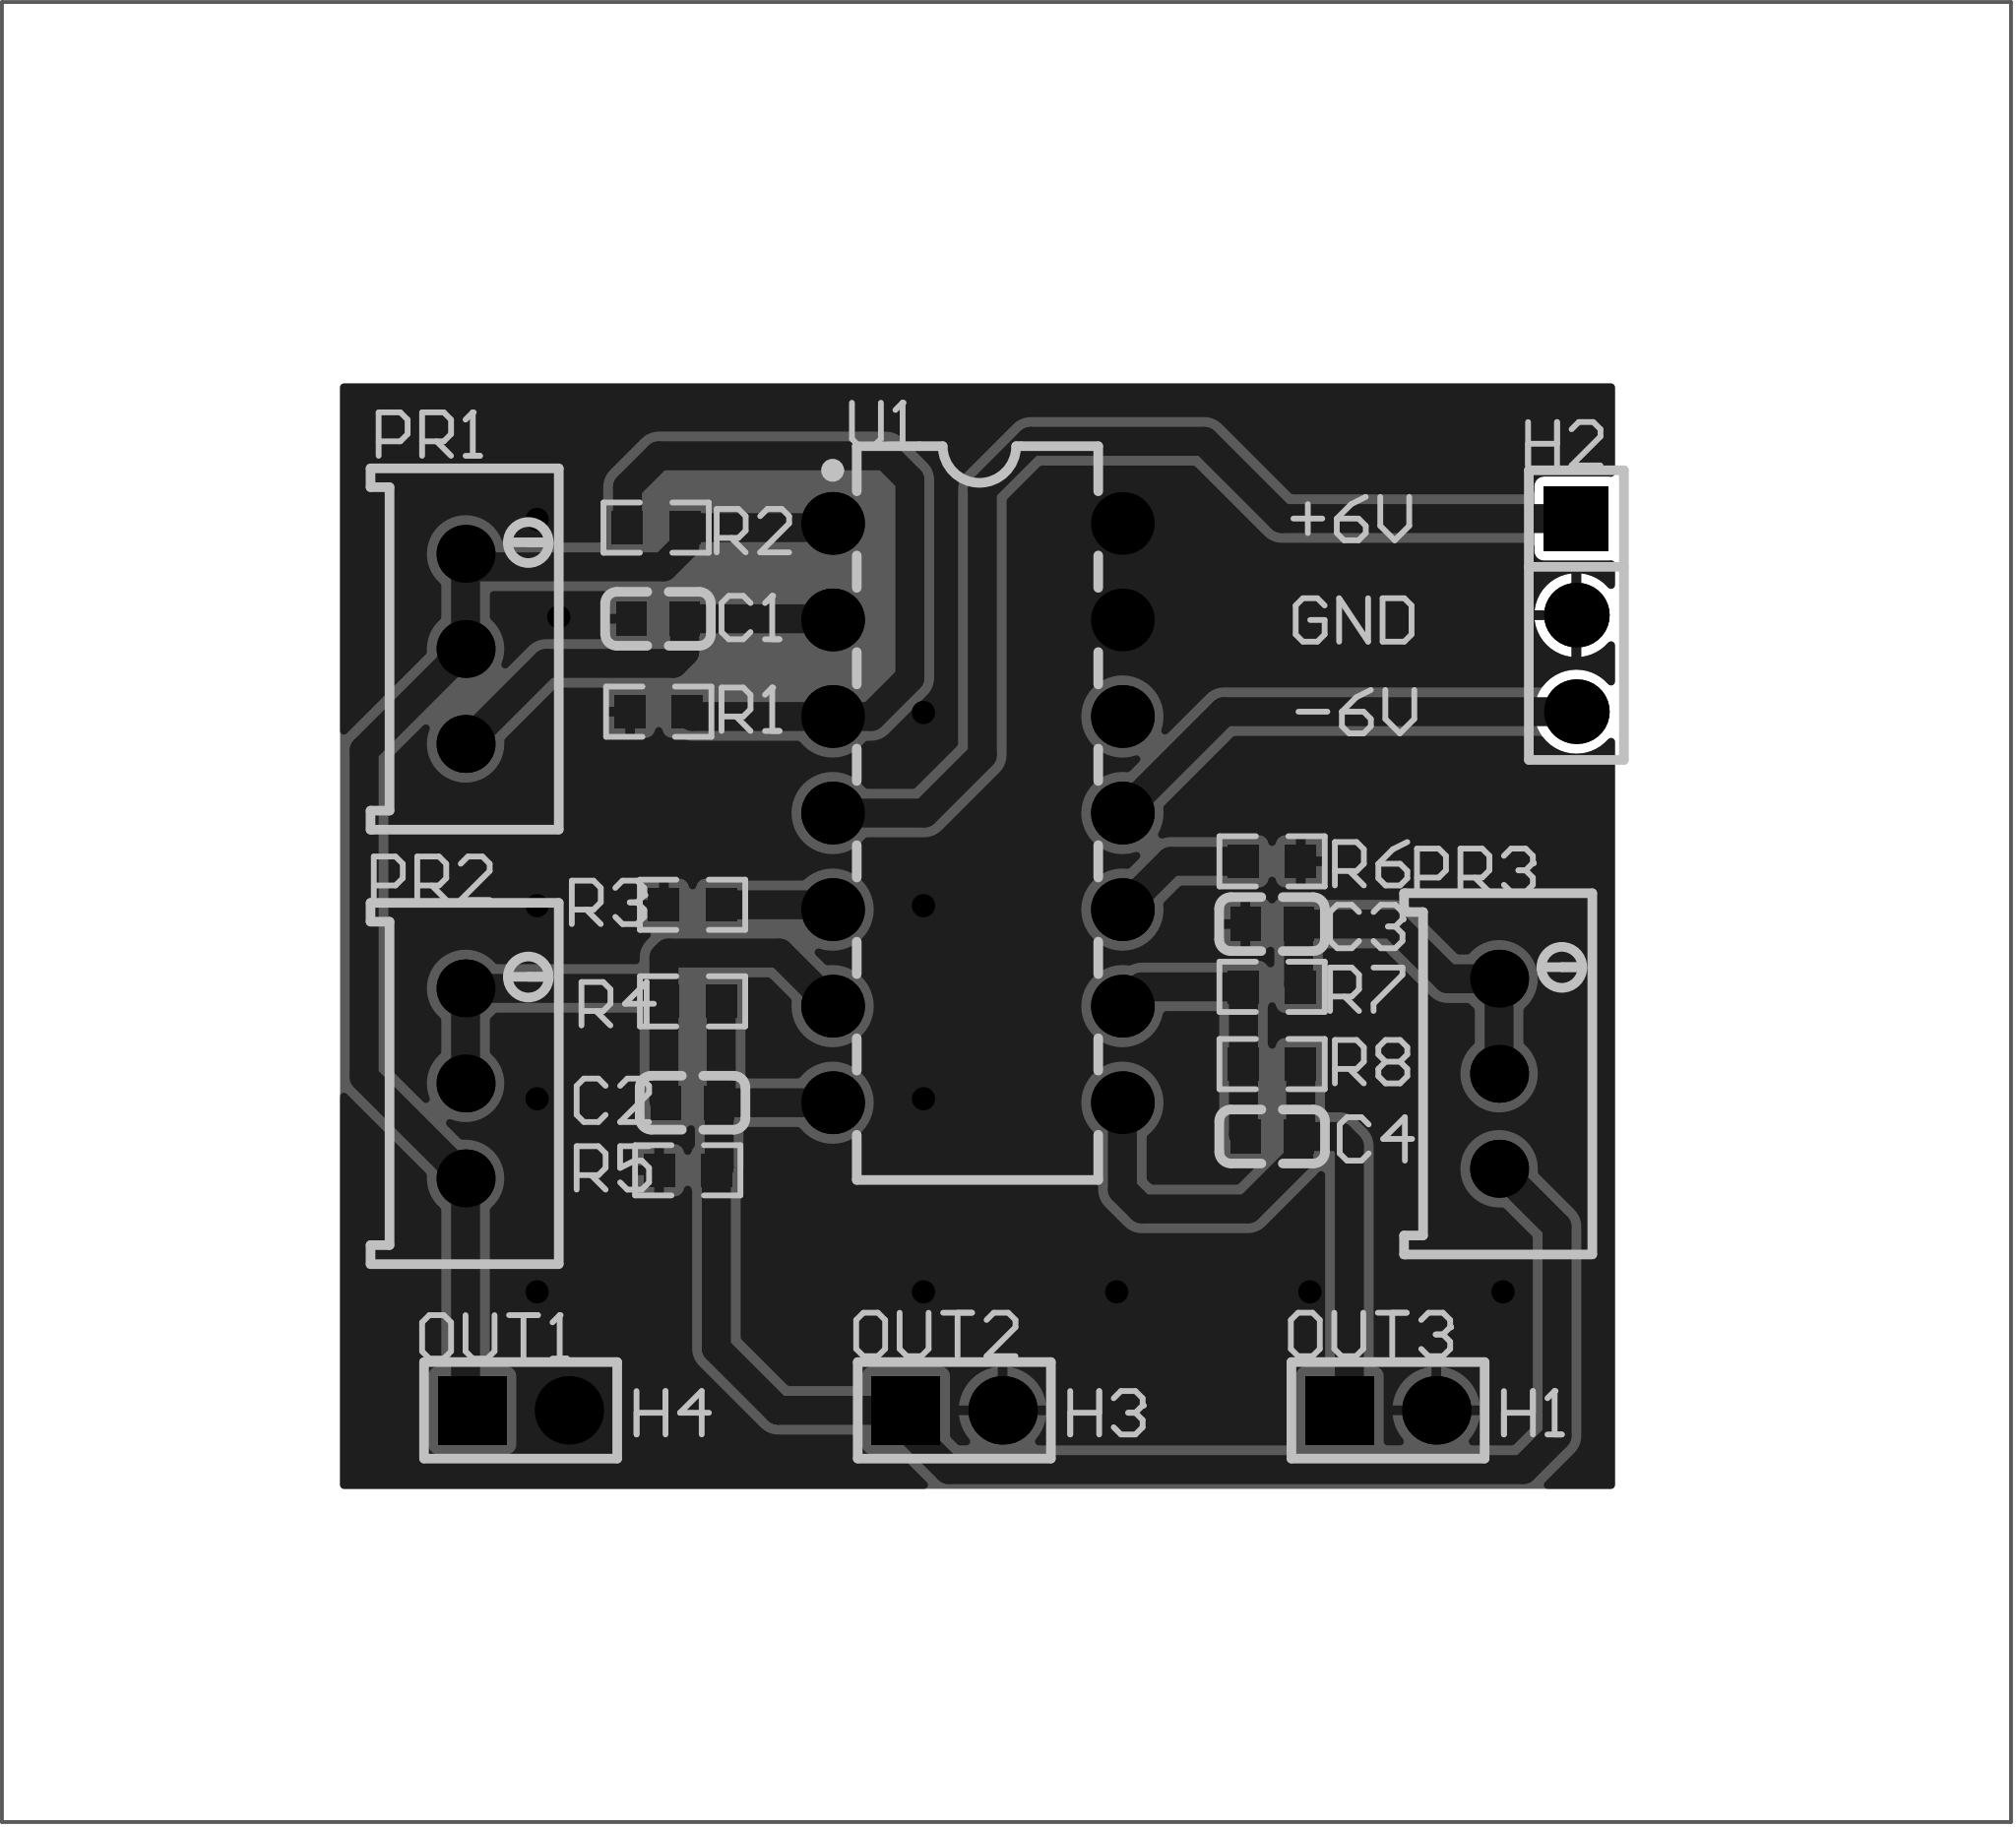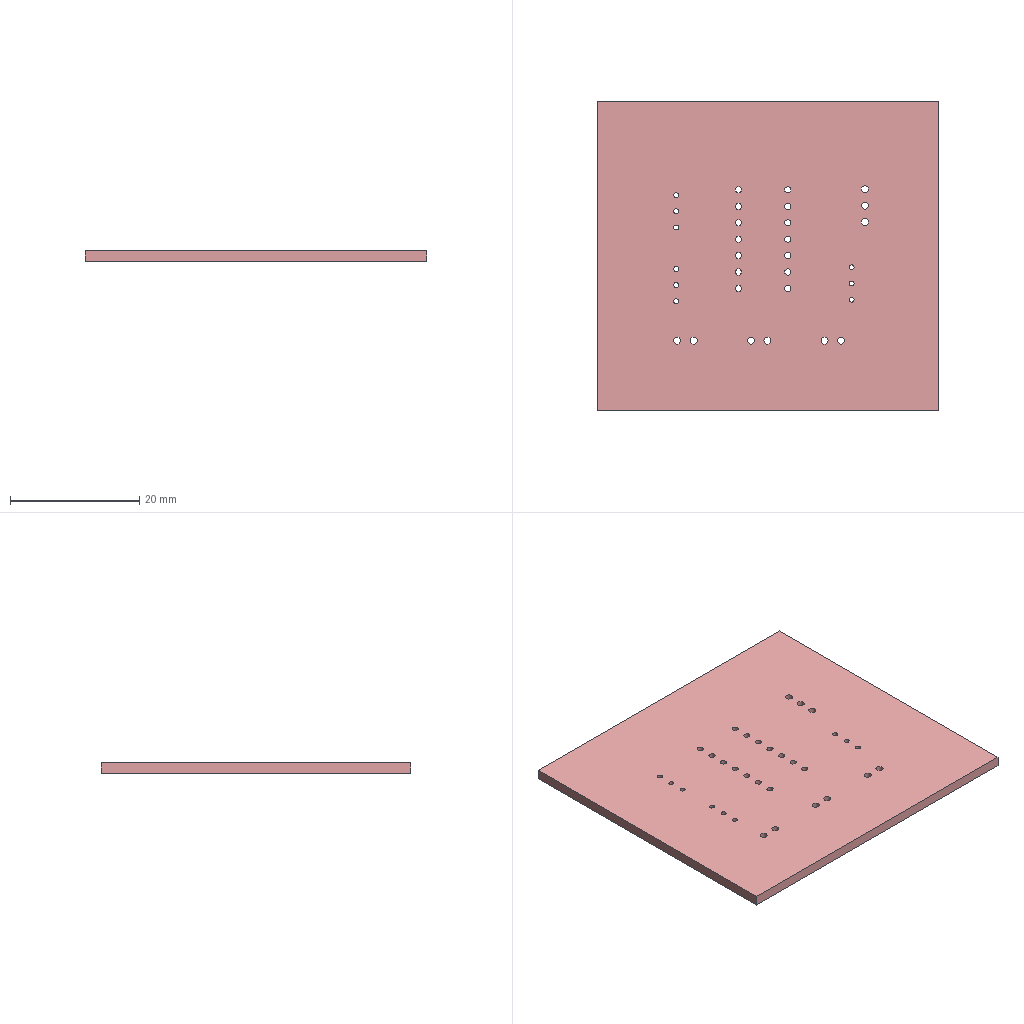Circuit board layout | Altium Designer | box 52.8 x 47.9 x 1.6 mm
Layer stack:
# Altium Designer layer stack of  (unit mm; dielectric type: 0 none, 1 core, 2 prepreg, 3 surface material)
index,name,kind,layer,copper_thickness_mm,dielectric_type,dielectric_thickness_mm,dielectric_material,dielectric_constant
0,Top Paste Mask Layer,other,,,,,,
1,Top Silkscreen Layer,other,,,,,,
2,Top Solder Mask Layer,dielectric,,,3,0.01,,3.3
3,Top Layer,copper,Top Layer,0.035,,,,
4,Dielectric1,dielectric,,,3,1.51,FR4,4.5
5,Bottom Layer,copper,Bottom Layer,0.035,,,,
6,Bottom Solder Mask Layer,dielectric,,,3,0.01,,3.3
7,Bottom Silkscreen Layer,other,,,,,,
8,Bottom Paste Mask Layer,other,,,,,,
# drill layer pairs: low layer,high layer
drill_pair,Top Layer,Bottom Layer
Part placement:
Designator,Comment,Layer,Footprint,Center-X(mm),Center-Y(mm),Rotation
C1,30nF,TopLayer,C0603,87.102,101.504,0
C2,100nF,TopLayer,C0603,88.011,88.773,0
C3,100nF,TopLayer,C0603,103.248,93.472,0
C4,100nF,TopLayer,C0603,103.251,87.884,0
H1,,TopLayer,HDR-TH_2P-P2.54-V-M-1,106.299,80.681,0
H2,,TopLayer,HDR-TH_3P-P2.54-V-M,111.252,101.6,270
PR1,10kΩ,TopLayer,R_3296,82.042,100.711,270
PR2,20kΩ,TopLayer,R_3296,82.042,89.281,270
PR3,200kΩ,TopLayer,R_3296,109.22,89.535,270
R1,10K,TopLayer,R0603,87.122,99.06,0
R2,3.9kΩ,TopLayer,R0603,87.053,103.902,180
R3,100K,TopLayer,R0603,88.011,93.98,0
R4,300K,TopLayer,R0603,88.011,91.44,0
R5,620,TopLayer,R0603,87.884,86.995,0
R6,10K,TopLayer,R0603,103.251,95.123,180
R7,20K,TopLayer,R0603,103.251,91.821,180
R8,24K,TopLayer,R0603,103.251,89.789,0
U1,LM324N/PB,TopLayer,PDIP-14_L19.2-W6.6-P2.54-LS7.6-BL,95.504,96.393,270
H3,,TopLayer,HDR-TH_2P-P2.54-V-M-1,94.894,80.681,0
H4,,TopLayer,HDR-TH_2P-P2.54-V-M-1,83.49,80.681,0
Pad and via stacks:
# Altium Designer via and pad stacks of  (unit mm). Each distinct definition once, with the count of objects using it.
# via: kind,start_layer,end_layer,hole_mm,diameter_mm,mode(0 simple;1 top-mid-bottom;2 full stack),diameter_per_layer,count,example_net
# pad: kind,layer,hole_mm,hole_type(0 round;1 square;2 slot),plating,top_size,top_shape(1 round;2 rect;3 octagon;9 rounded rect),mid_size,bottom_size,mode,footprint,size_per_layer,count,example
pad,Top Layer,0,0,plated,0.8x0.9,2,0.8x0.9,0.8x0.9,0,C0603,,8,C1.2
pad,Top Layer,0,0,plated,0.8065x0.864,2,0.8065x0.864,0.8065x0.864,0,R0603,,16,R1.2
pad,Multi-Layer,1.1,0,plated,1.8x1.8,1,1.8x1.8,1.8x1.8,0,HDR-TH_2P-P2.54-V-M-1,,3,H1.2
pad,Multi-Layer,1.1,0,plated,1.8x1.8,2,1.8x1.8,1.8x1.8,0,HDR-TH_2P-P2.54-V-M-1,,3,H1.1
pad,Multi-Layer,1.1,0,plated,1.7x1.7,2,1.7x1.7,1.7x1.7,0,HDR-TH_3P-P2.54-V-M,,1,H2.1
pad,Multi-Layer,1.1,0,plated,1.7x1.7,1,1.7x1.7,1.7x1.7,0,HDR-TH_3P-P2.54-V-M,,2,H2.2
pad,Multi-Layer,0.762,0,plated,1.524x1.524,1,1.524x1.524,1.524x1.524,0,R_3296,,9,PR1.2
pad,Multi-Layer,0.95,0,plated,1.65x1.65,1,1.65x1.65,1.65x1.65,0,PDIP-14_L19.2-W6.6-P2.54-LS7.6-BL,,14,U1.1
via,Top Layer,Bottom Layer,0.3048,0.61,0,,12,GND
Copper pours:
name,layer,net,type(0 solid;1 hatched;2 none)
Top Layer-GND,Top Layer,GND,0
Bottom Layer-GND,Bottom Layer,GND,0